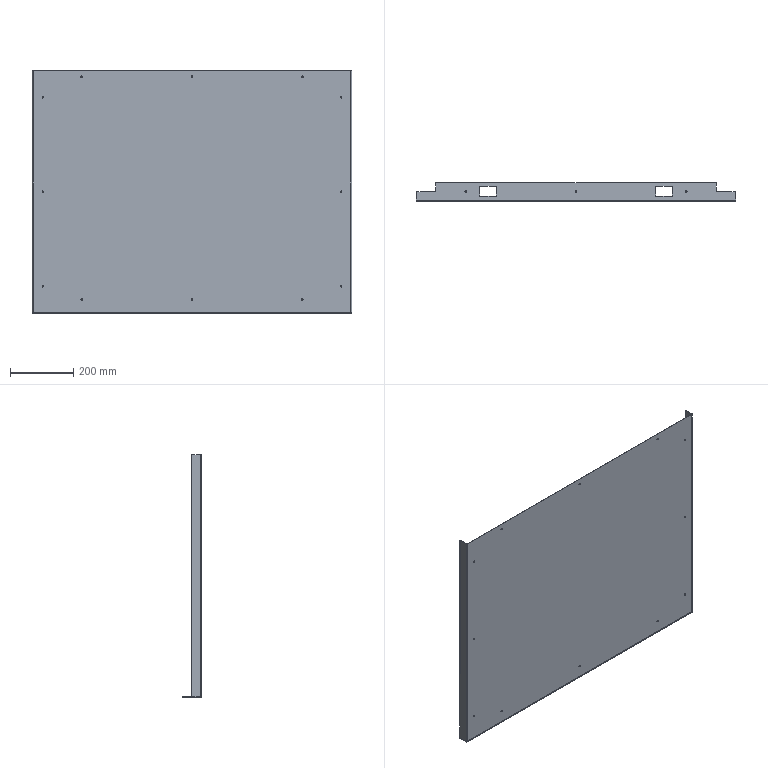Part | SolidWorks | features ICE 5, Fillet 3, Extrusion 1, Rip 1 | 1 solid | 64 faces | box 1013 x 60 x 770 mm | volume 1313614 mm3 | cylinder 36 | plane 28 | commonest cylinder face diameters 5 x30 3 x3 6 x3